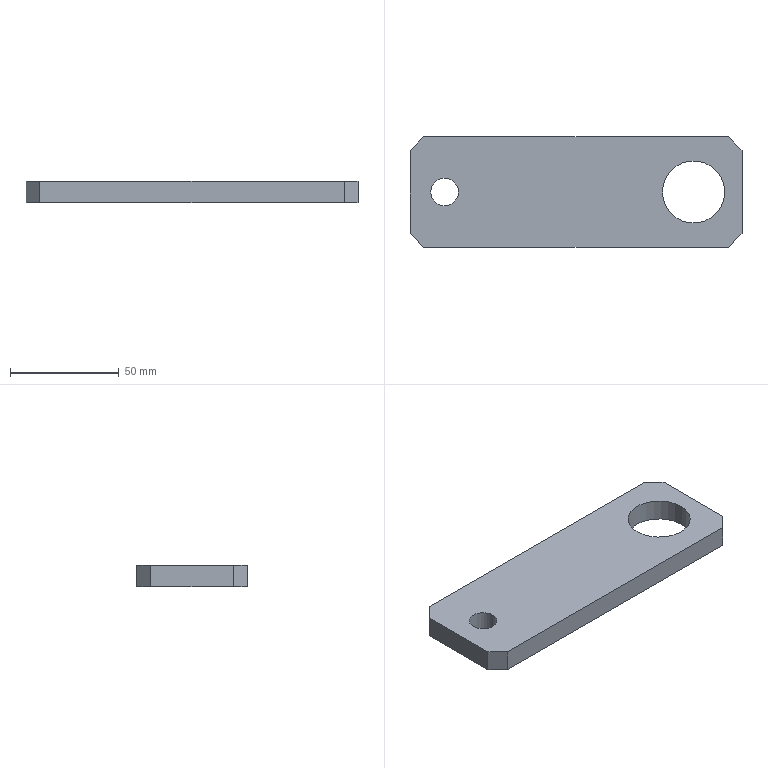Part | SolidWorks | features Chamfer 1, Extrusion 1 | 1 solid | 14 faces | box 152.4 x 50.8 x 10 mm | volume 68933 mm3 | plane 10 | cylinder 4 | commonest cylinder face diameters 12.7 x2 28.575 x2
STEP:
#1=CARTESIAN_POINT('',(-63.5,0.,5.));
#2=VERTEX_POINT('',#1);
#3=CARTESIAN_POINT('',(-50.8,0.,5.));
#4=VERTEX_POINT('',#3);
#5=CARTESIAN_POINT('',(-57.15,0.,5.));
#6=DIRECTION('',(0.,0.,1.));
#7=DIRECTION('',(1.,0.,0.));
#8=AXIS2_PLACEMENT_3D('',#5,#6,#7);
#9=CIRCLE('',#8,6.35);
#10=EDGE_CURVE('',#2,#4,#9,.T.);
#11=ORIENTED_EDGE('',*,*,#10,.T.);
#12=CARTESIAN_POINT('',(-50.8,0.,-5.));
#13=VERTEX_POINT('',#12);
#14=CARTESIAN_POINT('',(-50.8,0.,5.));
#15=DIRECTION('',(0.,0.,-1.));
#16=VECTOR('',#15,1000.);
#17=LINE('',#14,#16);
#18=EDGE_CURVE('',#4,#13,#17,.T.);
#19=ORIENTED_EDGE('',*,*,#18,.T.);
#20=CARTESIAN_POINT('',(-63.5,0.,-5.));
#21=VERTEX_POINT('',#20);
#22=CARTESIAN_POINT('',(-57.15,0.,-5.));
#23=DIRECTION('',(0.,0.,1.));
#24=DIRECTION('',(1.,0.,0.));
#25=AXIS2_PLACEMENT_3D('',#22,#23,#24);
#26=CIRCLE('',#25,6.35);
#27=EDGE_CURVE('',#21,#13,#26,.T.);
#28=ORIENTED_EDGE('',*,*,#27,.F.);
#29=CARTESIAN_POINT('',(-63.5,0.,5.));
#30=DIRECTION('',(0.,0.,-1.));
#31=VECTOR('',#30,1000.);
#32=LINE('',#29,#31);
#33=EDGE_CURVE('',#2,#21,#32,.T.);
#34=ORIENTED_EDGE('',*,*,#33,.F.);
#35=EDGE_LOOP('',(#11,#19,#28,#34));
#36=FACE_OUTER_BOUND('',#35,.T.);
#37=CARTESIAN_POINT('',(-57.15,0.,5.));
#38=DIRECTION('',(0.,0.,-1.));
#39=DIRECTION('',(-1.,0.,0.));
#40=AXIS2_PLACEMENT_3D('',#37,#38,#39);
#41=CYLINDRICAL_SURFACE('',#40,6.35);
#42=ADVANCED_FACE('',(#36),#41,.F.);
#43=CARTESIAN_POINT('',(42.863,0.,5.));
#44=VERTEX_POINT('',#43);
#45=CARTESIAN_POINT('',(71.438,0.,5.));
#46=VERTEX_POINT('',#45);
#47=CARTESIAN_POINT('',(57.15,0.,5.));
#48=DIRECTION('',(0.,0.,1.));
#49=DIRECTION('',(1.,0.,0.));
#50=AXIS2_PLACEMENT_3D('',#47,#48,#49);
#51=CIRCLE('',#50,14.288);
#52=EDGE_CURVE('',#44,#46,#51,.T.);
#53=ORIENTED_EDGE('',*,*,#52,.T.);
#54=CARTESIAN_POINT('',(71.438,0.,-5.));
#55=VERTEX_POINT('',#54);
#56=CARTESIAN_POINT('',(71.438,0.,5.));
#57=DIRECTION('',(0.,0.,-1.));
#58=VECTOR('',#57,1000.);
#59=LINE('',#56,#58);
#60=EDGE_CURVE('',#46,#55,#59,.T.);
#61=ORIENTED_EDGE('',*,*,#60,.T.);
#62=CARTESIAN_POINT('',(42.863,0.,-5.));
#63=VERTEX_POINT('',#62);
#64=CARTESIAN_POINT('',(57.15,0.,-5.));
#65=DIRECTION('',(0.,0.,1.));
#66=DIRECTION('',(1.,0.,0.));
#67=AXIS2_PLACEMENT_3D('',#64,#65,#66);
#68=CIRCLE('',#67,14.288);
#69=EDGE_CURVE('',#63,#55,#68,.T.);
#70=ORIENTED_EDGE('',*,*,#69,.F.);
#71=CARTESIAN_POINT('',(42.863,0.,5.));
#72=DIRECTION('',(0.,0.,-1.));
#73=VECTOR('',#72,1000.);
#74=LINE('',#71,#73);
#75=EDGE_CURVE('',#44,#63,#74,.T.);
#76=ORIENTED_EDGE('',*,*,#75,.F.);
#77=EDGE_LOOP('',(#53,#61,#70,#76));
#78=FACE_OUTER_BOUND('',#77,.T.);
#79=CARTESIAN_POINT('',(57.15,0.,5.));
#80=DIRECTION('',(0.,0.,-1.));
#81=DIRECTION('',(-1.,0.,0.));
#82=AXIS2_PLACEMENT_3D('',#79,#80,#81);
#83=CYLINDRICAL_SURFACE('',#82,14.288);
#84=ADVANCED_FACE('',(#78),#83,.F.);
#85=ORIENTED_EDGE('',*,*,#52,.F.);
#86=CARTESIAN_POINT('',(57.15,0.,5.));
#87=DIRECTION('',(0.,0.,1.));
#88=DIRECTION('',(1.,0.,0.));
#89=AXIS2_PLACEMENT_3D('',#86,#87,#88);
#90=CIRCLE('',#89,14.288);
#91=EDGE_CURVE('',#46,#44,#90,.T.);
#92=ORIENTED_EDGE('',*,*,#91,.F.);
#93=EDGE_LOOP('',(#85,#92));
#94=FACE_BOUND('',#93,.T.);
#95=CARTESIAN_POINT('',(-73.025,19.05,5.));
#96=VERTEX_POINT('',#95);
#97=CARTESIAN_POINT('',(-73.025,-19.05,5.));
#98=VERTEX_POINT('',#97);
#99=CARTESIAN_POINT('',(-73.025,25.4,5.));
#100=DIRECTION('',(0.,-1.,0.));
#101=VECTOR('',#100,1000.);
#102=LINE('',#99,#101);
#103=EDGE_CURVE('',#96,#98,#102,.T.);
#104=ORIENTED_EDGE('',*,*,#103,.T.);
#105=CARTESIAN_POINT('',(-66.675,-25.4,5.));
#106=VERTEX_POINT('',#105);
#107=CARTESIAN_POINT('',(-69.85,-22.225,5.));
#108=DIRECTION('',(0.7071,-0.7071,0.));
#109=VECTOR('',#108,1000.);
#110=LINE('',#107,#109);
#111=EDGE_CURVE('',#98,#106,#110,.T.);
#112=ORIENTED_EDGE('',*,*,#111,.T.);
#113=CARTESIAN_POINT('',(73.025,-25.4,5.));
#114=VERTEX_POINT('',#113);
#115=CARTESIAN_POINT('',(-73.025,-25.4,5.));
#116=DIRECTION('',(1.,0.,0.));
#117=VECTOR('',#116,1000.);
#118=LINE('',#115,#117);
#119=EDGE_CURVE('',#106,#114,#118,.T.);
#120=ORIENTED_EDGE('',*,*,#119,.T.);
#121=CARTESIAN_POINT('',(79.375,-19.05,5.));
#122=VERTEX_POINT('',#121);
#123=CARTESIAN_POINT('',(0.,-98.425,5.));
#124=DIRECTION('',(0.7071,0.7071,0.));
#125=VECTOR('',#124,1000.);
#126=LINE('',#123,#125);
#127=EDGE_CURVE('',#114,#122,#126,.T.);
#128=ORIENTED_EDGE('',*,*,#127,.T.);
#129=CARTESIAN_POINT('',(79.375,19.05,5.));
#130=VERTEX_POINT('',#129);
#131=CARTESIAN_POINT('',(79.375,25.4,5.));
#132=DIRECTION('',(0.,1.,0.));
#133=VECTOR('',#132,1000.);
#134=LINE('',#131,#133);
#135=EDGE_CURVE('',#122,#130,#134,.T.);
#136=ORIENTED_EDGE('',*,*,#135,.T.);
#137=CARTESIAN_POINT('',(73.025,25.4,5.));
#138=VERTEX_POINT('',#137);
#139=CARTESIAN_POINT('',(25.4,73.025,5.));
#140=DIRECTION('',(-0.7071,0.7071,0.));
#141=VECTOR('',#140,1000.);
#142=LINE('',#139,#141);
#143=EDGE_CURVE('',#130,#138,#142,.T.);
#144=ORIENTED_EDGE('',*,*,#143,.T.);
#145=CARTESIAN_POINT('',(-66.675,25.4,5.));
#146=VERTEX_POINT('',#145);
#147=CARTESIAN_POINT('',(-73.025,25.4,5.));
#148=DIRECTION('',(-1.,0.,0.));
#149=VECTOR('',#148,1000.);
#150=LINE('',#147,#149);
#151=EDGE_CURVE('',#138,#146,#150,.T.);
#152=ORIENTED_EDGE('',*,*,#151,.T.);
#153=CARTESIAN_POINT('',(-95.25,-3.175,5.));
#154=DIRECTION('',(-0.7071,-0.7071,0.));
#155=VECTOR('',#154,1000.);
#156=LINE('',#153,#155);
#157=EDGE_CURVE('',#146,#96,#156,.T.);
#158=ORIENTED_EDGE('',*,*,#157,.T.);
#159=EDGE_LOOP('',(#104,#112,#120,#128,#136,#144,#152,#158));
#160=FACE_OUTER_BOUND('',#159,.T.);
#161=ORIENTED_EDGE('',*,*,#10,.F.);
#162=CARTESIAN_POINT('',(-57.15,0.,5.));
#163=DIRECTION('',(0.,0.,1.));
#164=DIRECTION('',(1.,0.,0.));
#165=AXIS2_PLACEMENT_3D('',#162,#163,#164);
#166=CIRCLE('',#165,6.35);
#167=EDGE_CURVE('',#4,#2,#166,.T.);
#168=ORIENTED_EDGE('',*,*,#167,.F.);
#169=EDGE_LOOP('',(#161,#168));
#170=FACE_BOUND('',#169,.T.);
#171=CARTESIAN_POINT('',(-73.025,-25.4,5.));
#172=DIRECTION('',(0.,0.,1.));
#173=DIRECTION('',(1.,0.,0.));
#174=AXIS2_PLACEMENT_3D('',#171,#172,#173);
#175=PLANE('',#174);
#176=ADVANCED_FACE('',(#94,#160,#170),#175,.T.);
#177=ORIENTED_EDGE('',*,*,#69,.T.);
#178=CARTESIAN_POINT('',(57.15,0.,-5.));
#179=DIRECTION('',(0.,0.,1.));
#180=DIRECTION('',(1.,0.,0.));
#181=AXIS2_PLACEMENT_3D('',#178,#179,#180);
#182=CIRCLE('',#181,14.288);
#183=EDGE_CURVE('',#55,#63,#182,.T.);
#184=ORIENTED_EDGE('',*,*,#183,.T.);
#185=EDGE_LOOP('',(#177,#184));
#186=FACE_BOUND('',#185,.T.);
#187=CARTESIAN_POINT('',(-66.675,-25.4,-5.));
#188=VERTEX_POINT('',#187);
#189=CARTESIAN_POINT('',(73.025,-25.4,-5.));
#190=VERTEX_POINT('',#189);
#191=CARTESIAN_POINT('',(-73.025,-25.4,-5.));
#192=DIRECTION('',(1.,0.,0.));
#193=VECTOR('',#192,1000.);
#194=LINE('',#191,#193);
#195=EDGE_CURVE('',#188,#190,#194,.T.);
#196=ORIENTED_EDGE('',*,*,#195,.F.);
#197=CARTESIAN_POINT('',(-73.025,-19.05,-5.));
#198=VERTEX_POINT('',#197);
#199=CARTESIAN_POINT('',(-66.675,-25.4,-5.));
#200=DIRECTION('',(-0.7071,0.7071,0.));
#201=VECTOR('',#200,1000.);
#202=LINE('',#199,#201);
#203=EDGE_CURVE('',#188,#198,#202,.T.);
#204=ORIENTED_EDGE('',*,*,#203,.T.);
#205=CARTESIAN_POINT('',(-73.025,19.05,-5.));
#206=VERTEX_POINT('',#205);
#207=CARTESIAN_POINT('',(-73.025,25.4,-5.));
#208=DIRECTION('',(0.,-1.,0.));
#209=VECTOR('',#208,1000.);
#210=LINE('',#207,#209);
#211=EDGE_CURVE('',#206,#198,#210,.T.);
#212=ORIENTED_EDGE('',*,*,#211,.F.);
#213=CARTESIAN_POINT('',(-66.675,25.4,-5.));
#214=VERTEX_POINT('',#213);
#215=CARTESIAN_POINT('',(-73.025,19.05,-5.));
#216=DIRECTION('',(0.7071,0.7071,0.));
#217=VECTOR('',#216,1000.);
#218=LINE('',#215,#217);
#219=EDGE_CURVE('',#206,#214,#218,.T.);
#220=ORIENTED_EDGE('',*,*,#219,.T.);
#221=CARTESIAN_POINT('',(73.025,25.4,-5.));
#222=VERTEX_POINT('',#221);
#223=CARTESIAN_POINT('',(-73.025,25.4,-5.));
#224=DIRECTION('',(-1.,0.,0.));
#225=VECTOR('',#224,1000.);
#226=LINE('',#223,#225);
#227=EDGE_CURVE('',#222,#214,#226,.T.);
#228=ORIENTED_EDGE('',*,*,#227,.F.);
#229=CARTESIAN_POINT('',(79.375,19.05,-5.));
#230=VERTEX_POINT('',#229);
#231=CARTESIAN_POINT('',(73.025,25.4,-5.));
#232=DIRECTION('',(0.7071,-0.7071,0.));
#233=VECTOR('',#232,1000.);
#234=LINE('',#231,#233);
#235=EDGE_CURVE('',#222,#230,#234,.T.);
#236=ORIENTED_EDGE('',*,*,#235,.T.);
#237=CARTESIAN_POINT('',(79.375,-19.05,-5.));
#238=VERTEX_POINT('',#237);
#239=CARTESIAN_POINT('',(79.375,25.4,-5.));
#240=DIRECTION('',(0.,1.,0.));
#241=VECTOR('',#240,1000.);
#242=LINE('',#239,#241);
#243=EDGE_CURVE('',#238,#230,#242,.T.);
#244=ORIENTED_EDGE('',*,*,#243,.F.);
#245=CARTESIAN_POINT('',(79.375,-19.05,-5.));
#246=DIRECTION('',(-0.7071,-0.7071,0.));
#247=VECTOR('',#246,1000.);
#248=LINE('',#245,#247);
#249=EDGE_CURVE('',#238,#190,#248,.T.);
#250=ORIENTED_EDGE('',*,*,#249,.T.);
#251=EDGE_LOOP('',(#196,#204,#212,#220,#228,#236,#244,#250));
#252=FACE_OUTER_BOUND('',#251,.T.);
#253=ORIENTED_EDGE('',*,*,#27,.T.);
#254=CARTESIAN_POINT('',(-57.15,0.,-5.));
#255=DIRECTION('',(0.,0.,1.));
#256=DIRECTION('',(1.,0.,0.));
#257=AXIS2_PLACEMENT_3D('',#254,#255,#256);
#258=CIRCLE('',#257,6.35);
#259=EDGE_CURVE('',#13,#21,#258,.T.);
#260=ORIENTED_EDGE('',*,*,#259,.T.);
#261=EDGE_LOOP('',(#253,#260));
#262=FACE_BOUND('',#261,.T.);
#263=CARTESIAN_POINT('',(-73.025,-25.4,-5.));
#264=DIRECTION('',(0.,0.,1.));
#265=DIRECTION('',(1.,0.,0.));
#266=AXIS2_PLACEMENT_3D('',#263,#264,#265);
#267=PLANE('',#266);
#268=ADVANCED_FACE('',(#186,#252,#262),#267,.F.);
#269=ORIENTED_EDGE('',*,*,#211,.T.);
#270=CARTESIAN_POINT('',(-73.025,-19.05,5.));
#271=DIRECTION('',(0.,0.,1.));
#272=VECTOR('',#271,1000.);
#273=LINE('',#270,#272);
#274=EDGE_CURVE('',#198,#98,#273,.T.);
#275=ORIENTED_EDGE('',*,*,#274,.T.);
#276=ORIENTED_EDGE('',*,*,#103,.F.);
#277=CARTESIAN_POINT('',(-73.025,19.05,5.));
#278=DIRECTION('',(0.,0.,-1.));
#279=VECTOR('',#278,1000.);
#280=LINE('',#277,#279);
#281=EDGE_CURVE('',#96,#206,#280,.T.);
#282=ORIENTED_EDGE('',*,*,#281,.T.);
#283=EDGE_LOOP('',(#269,#275,#276,#282));
#284=FACE_OUTER_BOUND('',#283,.T.);
#285=CARTESIAN_POINT('',(-73.025,25.4,5.));
#286=DIRECTION('',(1.,0.,0.));
#287=DIRECTION('',(0.,0.,-1.));
#288=AXIS2_PLACEMENT_3D('',#285,#286,#287);
#289=PLANE('',#288);
#290=ADVANCED_FACE('',(#284),#289,.F.);
#291=ORIENTED_EDGE('',*,*,#119,.F.);
#292=CARTESIAN_POINT('',(-66.675,-25.4,5.));
#293=DIRECTION('',(0.,0.,-1.));
#294=VECTOR('',#293,1000.);
#295=LINE('',#292,#294);
#296=EDGE_CURVE('',#106,#188,#295,.T.);
#297=ORIENTED_EDGE('',*,*,#296,.T.);
#298=ORIENTED_EDGE('',*,*,#195,.T.);
#299=CARTESIAN_POINT('',(73.025,-25.4,5.));
#300=DIRECTION('',(0.,0.,1.));
#301=VECTOR('',#300,1000.);
#302=LINE('',#299,#301);
#303=EDGE_CURVE('',#190,#114,#302,.T.);
#304=ORIENTED_EDGE('',*,*,#303,.T.);
#305=EDGE_LOOP('',(#291,#297,#298,#304));
#306=FACE_OUTER_BOUND('',#305,.T.);
#307=CARTESIAN_POINT('',(-73.025,-25.4,5.));
#308=DIRECTION('',(0.,1.,0.));
#309=DIRECTION('',(-1.,0.,0.));
#310=AXIS2_PLACEMENT_3D('',#307,#308,#309);
#311=PLANE('',#310);
#312=ADVANCED_FACE('',(#306),#311,.F.);
#313=ORIENTED_EDGE('',*,*,#135,.F.);
#314=CARTESIAN_POINT('',(79.375,-19.05,5.));
#315=DIRECTION('',(0.,0.,-1.));
#316=VECTOR('',#315,1000.);
#317=LINE('',#314,#316);
#318=EDGE_CURVE('',#122,#238,#317,.T.);
#319=ORIENTED_EDGE('',*,*,#318,.T.);
#320=ORIENTED_EDGE('',*,*,#243,.T.);
#321=CARTESIAN_POINT('',(79.375,19.05,5.));
#322=DIRECTION('',(0.,0.,1.));
#323=VECTOR('',#322,1000.);
#324=LINE('',#321,#323);
#325=EDGE_CURVE('',#230,#130,#324,.T.);
#326=ORIENTED_EDGE('',*,*,#325,.T.);
#327=EDGE_LOOP('',(#313,#319,#320,#326));
#328=FACE_OUTER_BOUND('',#327,.T.);
#329=CARTESIAN_POINT('',(79.375,25.4,5.));
#330=DIRECTION('',(-1.,0.,0.));
#331=DIRECTION('',(0.,0.,1.));
#332=AXIS2_PLACEMENT_3D('',#329,#330,#331);
#333=PLANE('',#332);
#334=ADVANCED_FACE('',(#328),#333,.F.);
#335=ORIENTED_EDGE('',*,*,#227,.T.);
#336=CARTESIAN_POINT('',(-66.675,25.4,5.));
#337=DIRECTION('',(0.,0.,1.));
#338=VECTOR('',#337,1000.);
#339=LINE('',#336,#338);
#340=EDGE_CURVE('',#214,#146,#339,.T.);
#341=ORIENTED_EDGE('',*,*,#340,.T.);
#342=ORIENTED_EDGE('',*,*,#151,.F.);
#343=CARTESIAN_POINT('',(73.025,25.4,5.));
#344=DIRECTION('',(0.,0.,-1.));
#345=VECTOR('',#344,1000.);
#346=LINE('',#343,#345);
#347=EDGE_CURVE('',#138,#222,#346,.T.);
#348=ORIENTED_EDGE('',*,*,#347,.T.);
#349=EDGE_LOOP('',(#335,#341,#342,#348));
#350=FACE_OUTER_BOUND('',#349,.T.);
#351=CARTESIAN_POINT('',(-73.025,25.4,5.));
#352=DIRECTION('',(0.,-1.,0.));
#353=DIRECTION('',(1.,0.,0.));
#354=AXIS2_PLACEMENT_3D('',#351,#352,#353);
#355=PLANE('',#354);
#356=ADVANCED_FACE('',(#350),#355,.F.);
#357=ORIENTED_EDGE('',*,*,#60,.F.);
#358=ORIENTED_EDGE('',*,*,#91,.T.);
#359=ORIENTED_EDGE('',*,*,#75,.T.);
#360=ORIENTED_EDGE('',*,*,#183,.F.);
#361=EDGE_LOOP('',(#357,#358,#359,#360));
#362=FACE_OUTER_BOUND('',#361,.T.);
#363=CARTESIAN_POINT('',(57.15,0.,5.));
#364=DIRECTION('',(0.,0.,-1.));
#365=DIRECTION('',(-1.,0.,0.));
#366=AXIS2_PLACEMENT_3D('',#363,#364,#365);
#367=CYLINDRICAL_SURFACE('',#366,14.288);
#368=ADVANCED_FACE('',(#362),#367,.F.);
#369=ORIENTED_EDGE('',*,*,#18,.F.);
#370=ORIENTED_EDGE('',*,*,#167,.T.);
#371=ORIENTED_EDGE('',*,*,#33,.T.);
#372=ORIENTED_EDGE('',*,*,#259,.F.);
#373=EDGE_LOOP('',(#369,#370,#371,#372));
#374=FACE_OUTER_BOUND('',#373,.T.);
#375=CARTESIAN_POINT('',(-57.15,0.,5.));
#376=DIRECTION('',(0.,0.,-1.));
#377=DIRECTION('',(-1.,0.,0.));
#378=AXIS2_PLACEMENT_3D('',#375,#376,#377);
#379=CYLINDRICAL_SURFACE('',#378,6.35);
#380=ADVANCED_FACE('',(#374),#379,.F.);
#381=ORIENTED_EDGE('',*,*,#111,.F.);
#382=ORIENTED_EDGE('',*,*,#274,.F.);
#383=ORIENTED_EDGE('',*,*,#203,.F.);
#384=ORIENTED_EDGE('',*,*,#296,.F.);
#385=EDGE_LOOP('',(#381,#382,#383,#384));
#386=FACE_OUTER_BOUND('',#385,.T.);
#387=CARTESIAN_POINT('',(-66.675,-25.4,5.));
#388=DIRECTION('',(0.7071,0.7071,0.));
#389=DIRECTION('',(-0.7071,0.7071,0.));
#390=AXIS2_PLACEMENT_3D('',#387,#388,#389);
#391=PLANE('',#390);
#392=ADVANCED_FACE('',(#386),#391,.F.);
#393=ORIENTED_EDGE('',*,*,#157,.F.);
#394=ORIENTED_EDGE('',*,*,#340,.F.);
#395=ORIENTED_EDGE('',*,*,#219,.F.);
#396=ORIENTED_EDGE('',*,*,#281,.F.);
#397=EDGE_LOOP('',(#393,#394,#395,#396));
#398=FACE_OUTER_BOUND('',#397,.T.);
#399=CARTESIAN_POINT('',(-73.025,19.05,5.));
#400=DIRECTION('',(0.7071,-0.7071,0.));
#401=DIRECTION('',(0.7071,0.7071,0.));
#402=AXIS2_PLACEMENT_3D('',#399,#400,#401);
#403=PLANE('',#402);
#404=ADVANCED_FACE('',(#398),#403,.F.);
#405=ORIENTED_EDGE('',*,*,#127,.F.);
#406=ORIENTED_EDGE('',*,*,#303,.F.);
#407=ORIENTED_EDGE('',*,*,#249,.F.);
#408=ORIENTED_EDGE('',*,*,#318,.F.);
#409=EDGE_LOOP('',(#405,#406,#407,#408));
#410=FACE_OUTER_BOUND('',#409,.T.);
#411=CARTESIAN_POINT('',(79.375,-19.05,5.));
#412=DIRECTION('',(-0.7071,0.7071,0.));
#413=DIRECTION('',(-0.7071,-0.7071,0.));
#414=AXIS2_PLACEMENT_3D('',#411,#412,#413);
#415=PLANE('',#414);
#416=ADVANCED_FACE('',(#410),#415,.F.);
#417=ORIENTED_EDGE('',*,*,#143,.F.);
#418=ORIENTED_EDGE('',*,*,#325,.F.);
#419=ORIENTED_EDGE('',*,*,#235,.F.);
#420=ORIENTED_EDGE('',*,*,#347,.F.);
#421=EDGE_LOOP('',(#417,#418,#419,#420));
#422=FACE_OUTER_BOUND('',#421,.T.);
#423=CARTESIAN_POINT('',(73.025,25.4,5.));
#424=DIRECTION('',(-0.7071,-0.7071,0.));
#425=DIRECTION('',(0.7071,-0.7071,0.));
#426=AXIS2_PLACEMENT_3D('',#423,#424,#425);
#427=PLANE('',#426);
#428=ADVANCED_FACE('',(#422),#427,.F.);
#429=CLOSED_SHELL('',(#42,#84,#176,#268,#290,#312,#334,#356,#368,#380,#392,#404,#416,#428));
#430=MANIFOLD_SOLID_BREP('',#429);
#431=CARTESIAN_POINT('',(0.,0.,0.));
#432=DIRECTION('',(0.,0.,1.));
#433=DIRECTION('',(1.,0.,0.));
#434=AXIS2_PLACEMENT_3D('',#431,#432,#433);
#435=(LENGTH_UNIT()NAMED_UNIT(*)SI_UNIT(.MILLI.,.METRE.));
#436=UNCERTAINTY_MEASURE_WITH_UNIT(LENGTH_MEASURE(0.00001),#435,'','');
#437=(NAMED_UNIT(*)PLANE_ANGLE_UNIT()SI_UNIT($,.RADIAN.));
#438=(NAMED_UNIT(*)SI_UNIT($,.STERADIAN.)SOLID_ANGLE_UNIT());
#439=(GEOMETRIC_REPRESENTATION_CONTEXT(3)GLOBAL_UNCERTAINTY_ASSIGNED_CONTEXT((#436))GLOBAL_UNIT_ASSIGNED_CONTEXT((#435,#437,#438))REPRESENTATION_CONTEXT('',''));
#440=ADVANCED_BREP_SHAPE_REPRESENTATION('',(#430,#434),#439);